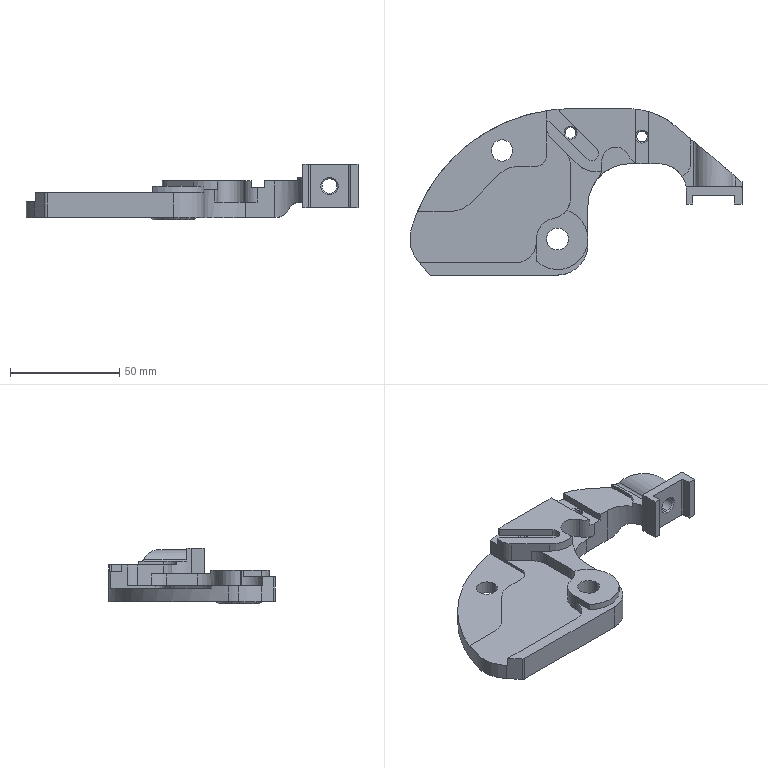Part | STEP file | MET_JAW_STD_ROT_GRM4 | 1 solid | 115 faces | box 152.146 x 76.2 x 25.425 mm | volume 65062 mm3 | cylinder 51 | plane 50 | cone 12 | spline 2 | commonest cylinder face diameters 12.7 x6 3.048 x5 19.304 x5 4.917 x4 25.4 x4 18.542 x3